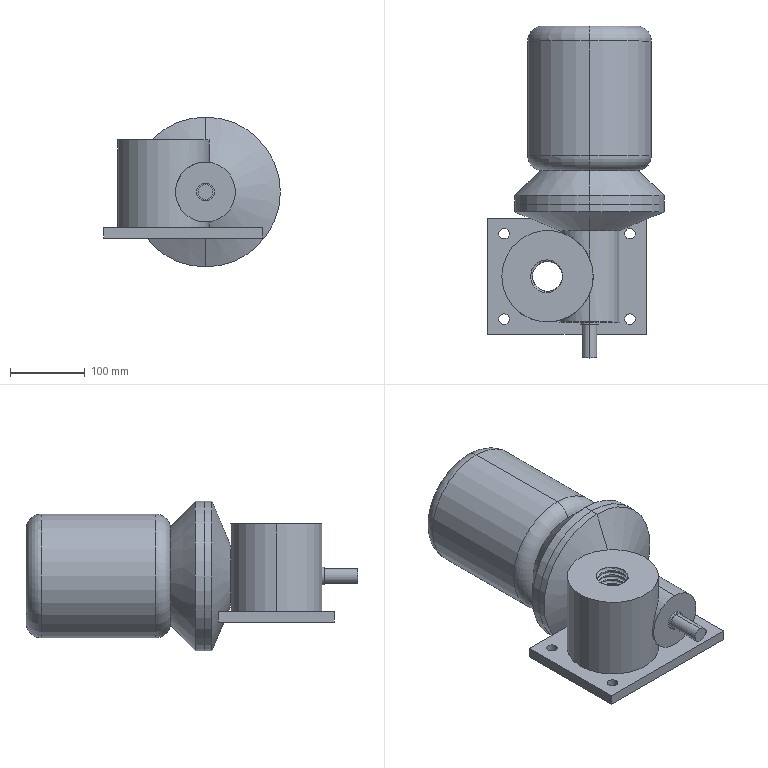Part | SolidWorks | features ICE 9, Blend 2, Fillet 2, Extrusion 1, Helix 1, RefAxis 1, SweepCut 1 | 3 solids | 79 faces | box 236 x 443.1 x 200 mm | volume 7884853 mm3 | cylinder 53 | plane 17 | cone 4 | torus 4 | spline 1 | commonest cylinder face diameters 40 x30 14 x8 200 x4 80 x3 20 x2 24 x2